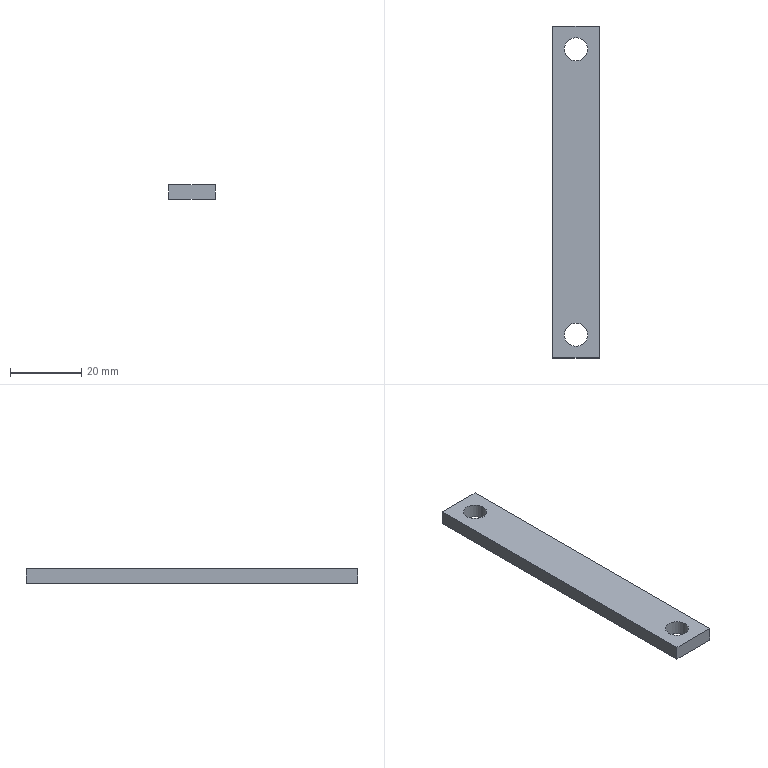Part | NX | features EXTRUDE 2, DATUM_CSYS 1, EXTRACT_DATUM_PLANE 1, SKETCH 1 | 1 solid | 8 faces | box 13 x 93 x 4 mm | volume 4571 mm3 | plane 6 | cylinder 2 | commonest cylinder face diameters 6.5 x2
STEP:
#1=CARTESIAN_POINT('',(6.5,46.5,0.));
#2=VERTEX_POINT('',#1);
#3=CARTESIAN_POINT('',(6.5,-46.5,0.));
#4=VERTEX_POINT('',#3);
#5=CARTESIAN_POINT('',(6.5,46.5,0.));
#6=DIRECTION('',(0.,-1.,0.));
#7=VECTOR('',#6,1000.);
#8=LINE('',#5,#7);
#9=EDGE_CURVE('',#2,#4,#8,.T.);
#10=ORIENTED_EDGE('',*,*,#9,.F.);
#11=CARTESIAN_POINT('',(6.5,46.5,4.));
#12=VERTEX_POINT('',#11);
#13=CARTESIAN_POINT('',(6.5,46.5,4.));
#14=DIRECTION('',(0.,0.,-1.));
#15=VECTOR('',#14,1000.);
#16=LINE('',#13,#15);
#17=EDGE_CURVE('',#12,#2,#16,.T.);
#18=ORIENTED_EDGE('',*,*,#17,.F.);
#19=CARTESIAN_POINT('',(6.5,-46.5,4.));
#20=VERTEX_POINT('',#19);
#21=CARTESIAN_POINT('',(6.5,46.5,4.));
#22=DIRECTION('',(0.,-1.,0.));
#23=VECTOR('',#22,1000.);
#24=LINE('',#21,#23);
#25=EDGE_CURVE('',#12,#20,#24,.T.);
#26=ORIENTED_EDGE('',*,*,#25,.T.);
#27=CARTESIAN_POINT('',(6.5,-46.5,4.));
#28=DIRECTION('',(0.,0.,-1.));
#29=VECTOR('',#28,1000.);
#30=LINE('',#27,#29);
#31=EDGE_CURVE('',#20,#4,#30,.T.);
#32=ORIENTED_EDGE('',*,*,#31,.T.);
#33=EDGE_LOOP('',(#10,#18,#26,#32));
#34=FACE_BOUND('',#33,.T.);
#35=CARTESIAN_POINT('',(6.5,46.5,4.));
#36=DIRECTION('',(1.,0.,0.));
#37=DIRECTION('',(0.,0.,-1.));
#38=AXIS2_PLACEMENT_3D('',#35,#36,#37);
#39=PLANE('',#38);
#40=ADVANCED_FACE('',(#34),#39,.T.);
#41=CARTESIAN_POINT('',(-6.5,-46.5,0.));
#42=VERTEX_POINT('',#41);
#43=CARTESIAN_POINT('',(6.5,-46.5,0.));
#44=DIRECTION('',(-1.,0.,0.));
#45=VECTOR('',#44,1000.);
#46=LINE('',#43,#45);
#47=EDGE_CURVE('',#4,#42,#46,.T.);
#48=ORIENTED_EDGE('',*,*,#47,.F.);
#49=ORIENTED_EDGE('',*,*,#31,.F.);
#50=CARTESIAN_POINT('',(-6.5,-46.5,4.));
#51=VERTEX_POINT('',#50);
#52=CARTESIAN_POINT('',(6.5,-46.5,4.));
#53=DIRECTION('',(-1.,0.,0.));
#54=VECTOR('',#53,1000.);
#55=LINE('',#52,#54);
#56=EDGE_CURVE('',#20,#51,#55,.T.);
#57=ORIENTED_EDGE('',*,*,#56,.T.);
#58=CARTESIAN_POINT('',(-6.5,-46.5,4.));
#59=DIRECTION('',(0.,0.,-1.));
#60=VECTOR('',#59,1000.);
#61=LINE('',#58,#60);
#62=EDGE_CURVE('',#51,#42,#61,.T.);
#63=ORIENTED_EDGE('',*,*,#62,.T.);
#64=EDGE_LOOP('',(#48,#49,#57,#63));
#65=FACE_BOUND('',#64,.T.);
#66=CARTESIAN_POINT('',(6.5,-46.5,4.));
#67=DIRECTION('',(0.,-1.,0.));
#68=DIRECTION('',(0.,0.,-1.));
#69=AXIS2_PLACEMENT_3D('',#66,#67,#68);
#70=PLANE('',#69);
#71=ADVANCED_FACE('',(#65),#70,.T.);
#72=CARTESIAN_POINT('',(-6.5,46.5,0.));
#73=VERTEX_POINT('',#72);
#74=CARTESIAN_POINT('',(-6.5,-46.5,0.));
#75=DIRECTION('',(0.,1.,0.));
#76=VECTOR('',#75,1000.);
#77=LINE('',#74,#76);
#78=EDGE_CURVE('',#42,#73,#77,.T.);
#79=ORIENTED_EDGE('',*,*,#78,.F.);
#80=ORIENTED_EDGE('',*,*,#62,.F.);
#81=CARTESIAN_POINT('',(-6.5,46.5,4.));
#82=VERTEX_POINT('',#81);
#83=CARTESIAN_POINT('',(-6.5,-46.5,4.));
#84=DIRECTION('',(0.,1.,0.));
#85=VECTOR('',#84,1000.);
#86=LINE('',#83,#85);
#87=EDGE_CURVE('',#51,#82,#86,.T.);
#88=ORIENTED_EDGE('',*,*,#87,.T.);
#89=CARTESIAN_POINT('',(-6.5,46.5,4.));
#90=DIRECTION('',(0.,0.,-1.));
#91=VECTOR('',#90,1000.);
#92=LINE('',#89,#91);
#93=EDGE_CURVE('',#82,#73,#92,.T.);
#94=ORIENTED_EDGE('',*,*,#93,.T.);
#95=EDGE_LOOP('',(#79,#80,#88,#94));
#96=FACE_BOUND('',#95,.T.);
#97=CARTESIAN_POINT('',(-6.5,-46.5,4.));
#98=DIRECTION('',(-1.,0.,0.));
#99=DIRECTION('',(0.,0.,1.));
#100=AXIS2_PLACEMENT_3D('',#97,#98,#99);
#101=PLANE('',#100);
#102=ADVANCED_FACE('',(#96),#101,.T.);
#103=CARTESIAN_POINT('',(-6.5,46.5,0.));
#104=DIRECTION('',(1.,0.,0.));
#105=VECTOR('',#104,1000.);
#106=LINE('',#103,#105);
#107=EDGE_CURVE('',#73,#2,#106,.T.);
#108=ORIENTED_EDGE('',*,*,#107,.F.);
#109=ORIENTED_EDGE('',*,*,#93,.F.);
#110=CARTESIAN_POINT('',(-6.5,46.5,4.));
#111=DIRECTION('',(1.,0.,0.));
#112=VECTOR('',#111,1000.);
#113=LINE('',#110,#112);
#114=EDGE_CURVE('',#82,#12,#113,.T.);
#115=ORIENTED_EDGE('',*,*,#114,.T.);
#116=ORIENTED_EDGE('',*,*,#17,.T.);
#117=EDGE_LOOP('',(#108,#109,#115,#116));
#118=FACE_BOUND('',#117,.T.);
#119=CARTESIAN_POINT('',(-6.5,46.5,4.));
#120=DIRECTION('',(0.,1.,0.));
#121=DIRECTION('',(0.,0.,1.));
#122=AXIS2_PLACEMENT_3D('',#119,#120,#121);
#123=PLANE('',#122);
#124=ADVANCED_FACE('',(#118),#123,.T.);
#125=CARTESIAN_POINT('',(3.25,40.,4.));
#126=VERTEX_POINT('',#125);
#127=CARTESIAN_POINT('',(0.,40.,4.));
#128=DIRECTION('',(0.,0.,1.));
#129=DIRECTION('',(1.,0.,0.));
#130=AXIS2_PLACEMENT_3D('',#127,#128,#129);
#131=CIRCLE('',#130,3.25);
#132=EDGE_CURVE('',#126,#126,#131,.T.);
#133=ORIENTED_EDGE('',*,*,#132,.F.);
#134=EDGE_LOOP('',(#133));
#135=FACE_BOUND('',#134,.T.);
#136=CARTESIAN_POINT('',(3.25,-40.,4.));
#137=VERTEX_POINT('',#136);
#138=CARTESIAN_POINT('',(0.,-40.,4.));
#139=DIRECTION('',(0.,0.,1.));
#140=DIRECTION('',(1.,0.,0.));
#141=AXIS2_PLACEMENT_3D('',#138,#139,#140);
#142=CIRCLE('',#141,3.25);
#143=EDGE_CURVE('',#137,#137,#142,.T.);
#144=ORIENTED_EDGE('',*,*,#143,.F.);
#145=EDGE_LOOP('',(#144));
#146=FACE_BOUND('',#145,.T.);
#147=ORIENTED_EDGE('',*,*,#25,.F.);
#148=ORIENTED_EDGE('',*,*,#114,.F.);
#149=ORIENTED_EDGE('',*,*,#87,.F.);
#150=ORIENTED_EDGE('',*,*,#56,.F.);
#151=EDGE_LOOP('',(#147,#148,#149,#150));
#152=FACE_BOUND('',#151,.T.);
#153=CARTESIAN_POINT('',(0.,0.,4.));
#154=DIRECTION('',(0.,0.,-1.));
#155=DIRECTION('',(-1.,0.,0.));
#156=AXIS2_PLACEMENT_3D('',#153,#154,#155);
#157=PLANE('',#156);
#158=ADVANCED_FACE('',(#135,#146,#152),#157,.F.);
#159=CARTESIAN_POINT('',(-3.25,40.,0.));
#160=VERTEX_POINT('',#159);
#161=CARTESIAN_POINT('',(0.,40.,0.));
#162=DIRECTION('',(0.,0.,1.));
#163=DIRECTION('',(-1.,0.,0.));
#164=AXIS2_PLACEMENT_3D('',#161,#162,#163);
#165=CIRCLE('',#164,3.25);
#166=EDGE_CURVE('',#160,#160,#165,.T.);
#167=ORIENTED_EDGE('',*,*,#166,.T.);
#168=EDGE_LOOP('',(#167));
#169=FACE_BOUND('',#168,.T.);
#170=CARTESIAN_POINT('',(-3.25,-40.,0.));
#171=VERTEX_POINT('',#170);
#172=CARTESIAN_POINT('',(0.,-40.,0.));
#173=DIRECTION('',(0.,0.,1.));
#174=DIRECTION('',(-1.,0.,0.));
#175=AXIS2_PLACEMENT_3D('',#172,#173,#174);
#176=CIRCLE('',#175,3.25);
#177=EDGE_CURVE('',#171,#171,#176,.T.);
#178=ORIENTED_EDGE('',*,*,#177,.T.);
#179=EDGE_LOOP('',(#178));
#180=FACE_BOUND('',#179,.T.);
#181=ORIENTED_EDGE('',*,*,#9,.T.);
#182=ORIENTED_EDGE('',*,*,#47,.T.);
#183=ORIENTED_EDGE('',*,*,#78,.T.);
#184=ORIENTED_EDGE('',*,*,#107,.T.);
#185=EDGE_LOOP('',(#181,#182,#183,#184));
#186=FACE_BOUND('',#185,.T.);
#187=CARTESIAN_POINT('',(0.,0.,0.));
#188=DIRECTION('',(0.,0.,-1.));
#189=DIRECTION('',(-1.,0.,0.));
#190=AXIS2_PLACEMENT_3D('',#187,#188,#189);
#191=PLANE('',#190);
#192=ADVANCED_FACE('',(#169,#180,#186),#191,.T.);
#193=ORIENTED_EDGE('',*,*,#177,.F.);
#194=EDGE_LOOP('',(#193));
#195=FACE_BOUND('',#194,.T.);
#196=ORIENTED_EDGE('',*,*,#143,.T.);
#197=EDGE_LOOP('',(#196));
#198=FACE_BOUND('',#197,.T.);
#199=CARTESIAN_POINT('',(0.,-40.,4.));
#200=DIRECTION('',(0.,0.,-1.));
#201=DIRECTION('',(-1.,0.,0.));
#202=AXIS2_PLACEMENT_3D('',#199,#200,#201);
#203=CYLINDRICAL_SURFACE('',#202,3.25);
#204=ADVANCED_FACE('',(#195,#198),#203,.F.);
#205=ORIENTED_EDGE('',*,*,#166,.F.);
#206=EDGE_LOOP('',(#205));
#207=FACE_BOUND('',#206,.T.);
#208=ORIENTED_EDGE('',*,*,#132,.T.);
#209=EDGE_LOOP('',(#208));
#210=FACE_BOUND('',#209,.T.);
#211=CARTESIAN_POINT('',(0.,40.,4.));
#212=DIRECTION('',(0.,0.,-1.));
#213=DIRECTION('',(-1.,0.,0.));
#214=AXIS2_PLACEMENT_3D('',#211,#212,#213);
#215=CYLINDRICAL_SURFACE('',#214,3.25);
#216=ADVANCED_FACE('',(#207,#210),#215,.F.);
#217=CLOSED_SHELL('',(#40,#71,#102,#124,#158,#192,#204,#216));
#218=MANIFOLD_SOLID_BREP('',#217);
#219=(LENGTH_UNIT()NAMED_UNIT(*)SI_UNIT(.MILLI.,.METRE.));
#220=UNCERTAINTY_MEASURE_WITH_UNIT(LENGTH_MEASURE(0.00001),#219,'','');
#221=(NAMED_UNIT(*)PLANE_ANGLE_UNIT()SI_UNIT($,.RADIAN.));
#222=(NAMED_UNIT(*)SI_UNIT($,.STERADIAN.)SOLID_ANGLE_UNIT());
#223=(GEOMETRIC_REPRESENTATION_CONTEXT(3)GLOBAL_UNCERTAINTY_ASSIGNED_CONTEXT((#220))GLOBAL_UNIT_ASSIGNED_CONTEXT((#219,#221,#222))REPRESENTATION_CONTEXT('',''));
#224=ADVANCED_BREP_SHAPE_REPRESENTATION('',(#218),#223);